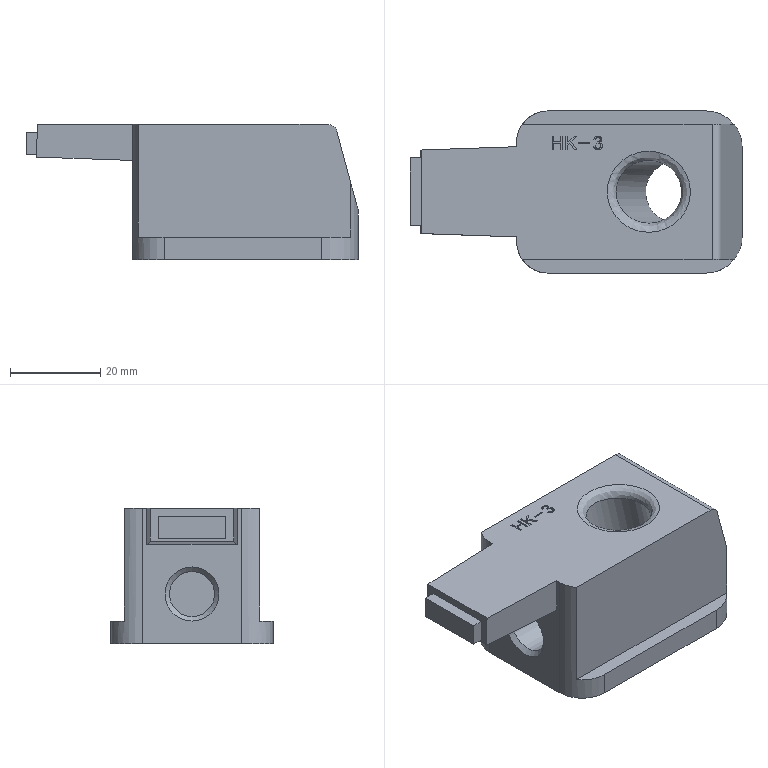Part | STEP file | solid 141 | 1 solid | 69 faces | box 73.616 x 36 x 30 mm | volume 41988 mm3 | plane 56 | cylinder 7 | other 4 | spline 1 | cone 1 | commonest cylinder face diameters 14 x3 16 x2 4 x1 10 x1